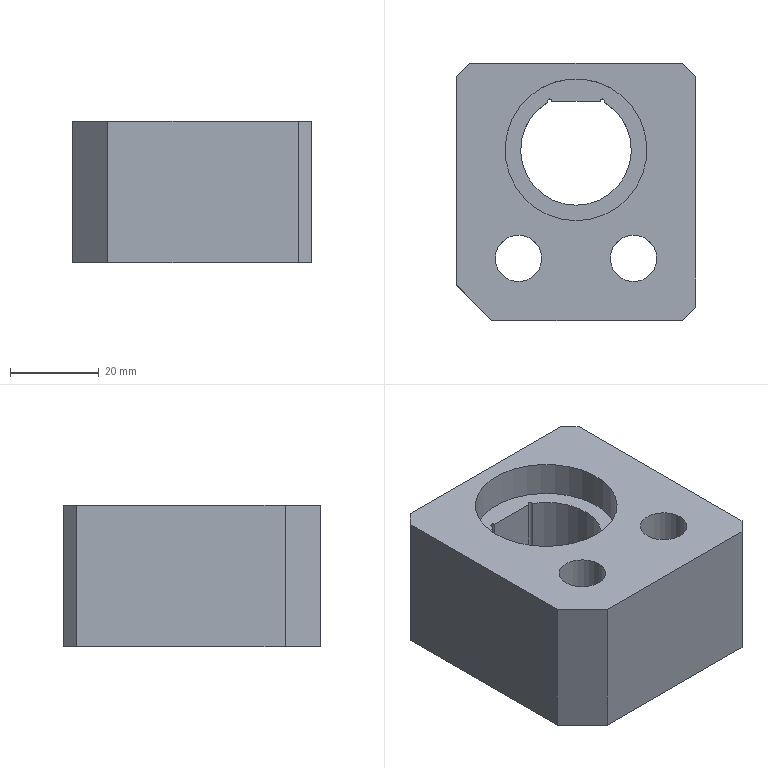Part | STEP file | lll_id3526_x_t | 1 solid | 23 faces | box 54 x 58 x 32 mm | volume 70505 mm3 | plane 14 | cylinder 9 | commonest cylinder face diameters 1 x2 10.5 x2 17 x2 25 x2 32 x1
STEP:
#1=CARTESIAN_POINT('',(3203.,139.5,84.5));
#2=VERTEX_POINT('',#1);
#3=CARTESIAN_POINT('',(3203.,155.5,84.5));
#4=DIRECTION('',(0.,0.,-1.));
#5=DIRECTION('',(1.,0.,0.));
#6=AXIS2_PLACEMENT_3D('',#3,#4,#5);
#7=CIRCLE('',#6,16.);
#8=EDGE_CURVE('',#2,#2,#7,.T.);
#9=ORIENTED_EDGE('',*,*,#8,.F.);
#10=EDGE_LOOP('',(#9));
#11=FACE_BOUND('',#10,.T.);
#12=CARTESIAN_POINT('',(3209.372,166.254,84.5));
#13=VERTEX_POINT('',#12);
#14=CARTESIAN_POINT('',(3208.437,166.5,84.5));
#15=VERTEX_POINT('',#14);
#16=CARTESIAN_POINT('',(3208.937,166.5,84.5));
#17=DIRECTION('',(0.,0.,1.));
#18=DIRECTION('',(-1.,0.,0.));
#19=AXIS2_PLACEMENT_3D('',#16,#17,#18);
#20=CIRCLE('',#19,0.5);
#21=EDGE_CURVE('',#13,#15,#20,.T.);
#22=ORIENTED_EDGE('',*,*,#21,.F.);
#23=CARTESIAN_POINT('',(3203.,143.,84.5));
#24=VERTEX_POINT('',#23);
#25=CARTESIAN_POINT('',(3203.,155.5,84.5));
#26=DIRECTION('',(0.,0.,1.));
#27=DIRECTION('',(0.,-1.,0.));
#28=AXIS2_PLACEMENT_3D('',#25,#26,#27);
#29=CIRCLE('',#28,12.5);
#30=EDGE_CURVE('',#24,#13,#29,.T.);
#31=ORIENTED_EDGE('',*,*,#30,.F.);
#32=CARTESIAN_POINT('',(3196.628,166.254,84.5));
#33=VERTEX_POINT('',#32);
#34=CARTESIAN_POINT('',(3203.,155.5,84.5));
#35=DIRECTION('',(0.,0.,1.));
#36=DIRECTION('',(0.,-1.,0.));
#37=AXIS2_PLACEMENT_3D('',#34,#35,#36);
#38=CIRCLE('',#37,12.5);
#39=EDGE_CURVE('',#33,#24,#38,.T.);
#40=ORIENTED_EDGE('',*,*,#39,.F.);
#41=CARTESIAN_POINT('',(3197.563,166.5,84.5));
#42=VERTEX_POINT('',#41);
#43=CARTESIAN_POINT('',(3197.063,166.5,84.5));
#44=DIRECTION('',(0.,0.,-1.));
#45=DIRECTION('',(1.,0.,0.));
#46=AXIS2_PLACEMENT_3D('',#43,#44,#45);
#47=CIRCLE('',#46,0.5);
#48=EDGE_CURVE('',#33,#42,#47,.T.);
#49=ORIENTED_EDGE('',*,*,#48,.T.);
#50=CARTESIAN_POINT('',(3203.,166.5,84.5));
#51=DIRECTION('',(1.,0.,0.));
#52=VECTOR('',#51,1.);
#53=LINE('',#50,#52);
#54=EDGE_CURVE('',#42,#15,#53,.T.);
#55=ORIENTED_EDGE('',*,*,#54,.T.);
#56=EDGE_LOOP('',(#22,#31,#40,#49,#55));
#57=FACE_BOUND('',#56,.T.);
#58=CARTESIAN_POINT('',(3203.,141.75,84.5));
#59=DIRECTION('',(0.,0.,-1.));
#60=DIRECTION('',(0.,-1.,0.));
#61=AXIS2_PLACEMENT_3D('',#58,#59,#60);
#62=PLANE('',#61);
#63=ADVANCED_FACE('',(#11,#57),#62,.F.);
#64=CARTESIAN_POINT('',(3210.75,131.,77.5));
#65=VERTEX_POINT('',#64);
#66=CARTESIAN_POINT('',(3216.,131.,77.5));
#67=DIRECTION('',(0.,0.,1.));
#68=DIRECTION('',(-1.,0.,0.));
#69=AXIS2_PLACEMENT_3D('',#66,#67,#68);
#70=CIRCLE('',#69,5.25);
#71=EDGE_CURVE('',#65,#65,#70,.T.);
#72=ORIENTED_EDGE('',*,*,#71,.T.);
#73=EDGE_LOOP('',(#72));
#74=FACE_BOUND('',#73,.T.);
#75=CARTESIAN_POINT('',(3207.5,131.,77.5));
#76=VERTEX_POINT('',#75);
#77=CARTESIAN_POINT('',(3216.,131.,77.5));
#78=DIRECTION('',(0.,0.,1.));
#79=DIRECTION('',(-1.,0.,0.));
#80=AXIS2_PLACEMENT_3D('',#77,#78,#79);
#81=CIRCLE('',#80,8.5);
#82=EDGE_CURVE('',#76,#76,#81,.T.);
#83=ORIENTED_EDGE('',*,*,#82,.F.);
#84=EDGE_LOOP('',(#83));
#85=FACE_BOUND('',#84,.T.);
#86=CARTESIAN_POINT('',(3216.,131.,77.5));
#87=DIRECTION('',(0.,0.,1.));
#88=DIRECTION('',(1.,0.,0.));
#89=AXIS2_PLACEMENT_3D('',#86,#87,#88);
#90=PLANE('',#89);
#91=ADVANCED_FACE('',(#74,#85),#90,.F.);
#92=ORIENTED_EDGE('',*,*,#82,.T.);
#93=EDGE_LOOP('',(#92));
#94=FACE_BOUND('',#93,.T.);
#95=CARTESIAN_POINT('',(3207.5,131.,60.5));
#96=VERTEX_POINT('',#95);
#97=CARTESIAN_POINT('',(3216.,131.,60.5));
#98=DIRECTION('',(0.,0.,-1.));
#99=DIRECTION('',(-1.,0.,0.));
#100=AXIS2_PLACEMENT_3D('',#97,#98,#99);
#101=CIRCLE('',#100,8.5);
#102=EDGE_CURVE('',#96,#96,#101,.T.);
#103=ORIENTED_EDGE('',*,*,#102,.T.);
#104=EDGE_LOOP('',(#103));
#105=FACE_BOUND('',#104,.T.);
#106=CARTESIAN_POINT('',(3216.,131.,60.5));
#107=DIRECTION('',(0.,0.,1.));
#108=DIRECTION('',(1.,0.,0.));
#109=AXIS2_PLACEMENT_3D('',#106,#107,#108);
#110=CYLINDRICAL_SURFACE('',#109,8.5);
#111=ADVANCED_FACE('',(#94,#105),#110,.F.);
#112=CARTESIAN_POINT('',(3176.,172.,60.5));
#113=VERTEX_POINT('',#112);
#114=CARTESIAN_POINT('',(3179.,175.,60.5));
#115=VERTEX_POINT('',#114);
#116=CARTESIAN_POINT('',(3196.207,192.207,60.5));
#117=DIRECTION('',(0.7071,0.7071,0.));
#118=VECTOR('',#117,1.);
#119=LINE('',#116,#118);
#120=EDGE_CURVE('',#113,#115,#119,.T.);
#121=ORIENTED_EDGE('',*,*,#120,.F.);
#122=CARTESIAN_POINT('',(3176.,172.,92.5));
#123=VERTEX_POINT('',#122);
#124=CARTESIAN_POINT('',(3176.,172.,-8.5));
#125=DIRECTION('',(0.,0.,-1.));
#126=VECTOR('',#125,1.);
#127=LINE('',#124,#126);
#128=EDGE_CURVE('',#123,#113,#127,.T.);
#129=ORIENTED_EDGE('',*,*,#128,.F.);
#130=CARTESIAN_POINT('',(3179.,175.,92.5));
#131=VERTEX_POINT('',#130);
#132=CARTESIAN_POINT('',(3196.207,192.207,92.5));
#133=DIRECTION('',(-0.7071,-0.7071,0.));
#134=VECTOR('',#133,1.);
#135=LINE('',#132,#134);
#136=EDGE_CURVE('',#131,#123,#135,.T.);
#137=ORIENTED_EDGE('',*,*,#136,.F.);
#138=CARTESIAN_POINT('',(3179.,175.,-8.5));
#139=DIRECTION('',(0.,0.,1.));
#140=VECTOR('',#139,1.);
#141=LINE('',#138,#140);
#142=EDGE_CURVE('',#115,#131,#141,.T.);
#143=ORIENTED_EDGE('',*,*,#142,.F.);
#144=EDGE_LOOP('',(#121,#129,#137,#143));
#145=FACE_OUTER_BOUND('',#144,.T.);
#146=CARTESIAN_POINT('',(3179.,175.,-8.5));
#147=DIRECTION('',(0.7071,-0.7071,0.));
#148=DIRECTION('',(0.,0.,1.));
#149=AXIS2_PLACEMENT_3D('',#146,#147,#148);
#150=PLANE('',#149);
#151=ADVANCED_FACE('',(#145),#150,.F.);
#152=CARTESIAN_POINT('',(3227.,175.,60.5));
#153=VERTEX_POINT('',#152);
#154=CARTESIAN_POINT('',(3271.14,175.,60.5));
#155=DIRECTION('',(1.,0.,0.));
#156=VECTOR('',#155,1.);
#157=LINE('',#154,#156);
#158=EDGE_CURVE('',#115,#153,#157,.T.);
#159=ORIENTED_EDGE('',*,*,#158,.F.);
#160=ORIENTED_EDGE('',*,*,#142,.T.);
#161=CARTESIAN_POINT('',(3227.,175.,92.5));
#162=VERTEX_POINT('',#161);
#163=CARTESIAN_POINT('',(3271.14,175.,92.5));
#164=DIRECTION('',(-1.,0.,0.));
#165=VECTOR('',#164,1.);
#166=LINE('',#163,#165);
#167=EDGE_CURVE('',#162,#131,#166,.T.);
#168=ORIENTED_EDGE('',*,*,#167,.F.);
#169=CARTESIAN_POINT('',(3227.,175.,-8.5));
#170=DIRECTION('',(0.,0.,-1.));
#171=VECTOR('',#170,1.);
#172=LINE('',#169,#171);
#173=EDGE_CURVE('',#162,#153,#172,.T.);
#174=ORIENTED_EDGE('',*,*,#173,.T.);
#175=EDGE_LOOP('',(#159,#160,#168,#174));
#176=FACE_OUTER_BOUND('',#175,.T.);
#177=CARTESIAN_POINT('',(3203.,175.,-8.5));
#178=DIRECTION('',(0.,1.,0.));
#179=DIRECTION('',(0.,0.,-1.));
#180=AXIS2_PLACEMENT_3D('',#177,#178,#179);
#181=PLANE('',#180);
#182=ADVANCED_FACE('',(#176),#181,.T.);
#183=CARTESIAN_POINT('',(3230.,172.,60.5));
#184=VERTEX_POINT('',#183);
#185=CARTESIAN_POINT('',(3277.933,124.067,60.5));
#186=DIRECTION('',(0.7071,-0.7071,0.));
#187=VECTOR('',#186,1.);
#188=LINE('',#185,#187);
#189=EDGE_CURVE('',#153,#184,#188,.T.);
#190=ORIENTED_EDGE('',*,*,#189,.F.);
#191=ORIENTED_EDGE('',*,*,#173,.F.);
#192=CARTESIAN_POINT('',(3230.,172.,92.5));
#193=VERTEX_POINT('',#192);
#194=CARTESIAN_POINT('',(3277.933,124.067,92.5));
#195=DIRECTION('',(-0.7071,0.7071,0.));
#196=VECTOR('',#195,1.);
#197=LINE('',#194,#196);
#198=EDGE_CURVE('',#193,#162,#197,.T.);
#199=ORIENTED_EDGE('',*,*,#198,.F.);
#200=CARTESIAN_POINT('',(3230.,172.,-8.5));
#201=DIRECTION('',(0.,0.,1.));
#202=VECTOR('',#201,1.);
#203=LINE('',#200,#202);
#204=EDGE_CURVE('',#184,#193,#203,.T.);
#205=ORIENTED_EDGE('',*,*,#204,.F.);
#206=EDGE_LOOP('',(#190,#191,#199,#205));
#207=FACE_OUTER_BOUND('',#206,.T.);
#208=CARTESIAN_POINT('',(3230.,172.,-8.5));
#209=DIRECTION('',(-0.7071,-0.7071,0.));
#210=DIRECTION('',(0.,0.,1.));
#211=AXIS2_PLACEMENT_3D('',#208,#209,#210);
#212=PLANE('',#211);
#213=ADVANCED_FACE('',(#207),#212,.F.);
#214=CARTESIAN_POINT('',(3230.,120.,92.5));
#215=VERTEX_POINT('',#214);
#216=CARTESIAN_POINT('',(3230.,124.275,92.5));
#217=DIRECTION('',(0.,1.,0.));
#218=VECTOR('',#217,1.);
#219=LINE('',#216,#218);
#220=EDGE_CURVE('',#215,#193,#219,.T.);
#221=ORIENTED_EDGE('',*,*,#220,.F.);
#222=CARTESIAN_POINT('',(3230.,120.,60.5));
#223=VERTEX_POINT('',#222);
#224=CARTESIAN_POINT('',(3230.,120.,-8.5));
#225=DIRECTION('',(0.,0.,-1.));
#226=VECTOR('',#225,1.);
#227=LINE('',#224,#226);
#228=EDGE_CURVE('',#215,#223,#227,.T.);
#229=ORIENTED_EDGE('',*,*,#228,.T.);
#230=CARTESIAN_POINT('',(3230.,124.275,60.5));
#231=DIRECTION('',(0.,-1.,0.));
#232=VECTOR('',#231,1.);
#233=LINE('',#230,#232);
#234=EDGE_CURVE('',#184,#223,#233,.T.);
#235=ORIENTED_EDGE('',*,*,#234,.F.);
#236=ORIENTED_EDGE('',*,*,#204,.T.);
#237=EDGE_LOOP('',(#221,#229,#235,#236));
#238=FACE_OUTER_BOUND('',#237,.T.);
#239=CARTESIAN_POINT('',(3230.,155.5,-8.5));
#240=DIRECTION('',(1.,0.,0.));
#241=DIRECTION('',(0.,0.,-1.));
#242=AXIS2_PLACEMENT_3D('',#239,#240,#241);
#243=PLANE('',#242);
#244=ADVANCED_FACE('',(#238),#243,.T.);
#245=CARTESIAN_POINT('',(3227.,117.,60.5));
#246=VERTEX_POINT('',#245);
#247=CARTESIAN_POINT('',(3256.207,146.207,60.5));
#248=DIRECTION('',(-0.7071,-0.7071,0.));
#249=VECTOR('',#248,1.);
#250=LINE('',#247,#249);
#251=EDGE_CURVE('',#223,#246,#250,.T.);
#252=ORIENTED_EDGE('',*,*,#251,.F.);
#253=ORIENTED_EDGE('',*,*,#228,.F.);
#254=CARTESIAN_POINT('',(3227.,117.,92.5));
#255=VERTEX_POINT('',#254);
#256=CARTESIAN_POINT('',(3256.207,146.207,92.5));
#257=DIRECTION('',(0.7071,0.7071,0.));
#258=VECTOR('',#257,1.);
#259=LINE('',#256,#258);
#260=EDGE_CURVE('',#255,#215,#259,.T.);
#261=ORIENTED_EDGE('',*,*,#260,.F.);
#262=CARTESIAN_POINT('',(3227.,117.,-8.5));
#263=DIRECTION('',(0.,0.,1.));
#264=VECTOR('',#263,1.);
#265=LINE('',#262,#264);
#266=EDGE_CURVE('',#246,#255,#265,.T.);
#267=ORIENTED_EDGE('',*,*,#266,.F.);
#268=EDGE_LOOP('',(#252,#253,#261,#267));
#269=FACE_OUTER_BOUND('',#268,.T.);
#270=CARTESIAN_POINT('',(3227.,117.,-8.5));
#271=DIRECTION('',(-0.7071,0.7071,0.));
#272=DIRECTION('',(0.,0.,1.));
#273=AXIS2_PLACEMENT_3D('',#270,#271,#272);
#274=PLANE('',#273);
#275=ADVANCED_FACE('',(#269),#274,.F.);
#276=CARTESIAN_POINT('',(3184.,117.,92.5));
#277=VERTEX_POINT('',#276);
#278=CARTESIAN_POINT('',(3271.14,117.,92.5));
#279=DIRECTION('',(1.,0.,0.));
#280=VECTOR('',#279,1.);
#281=LINE('',#278,#280);
#282=EDGE_CURVE('',#277,#255,#281,.T.);
#283=ORIENTED_EDGE('',*,*,#282,.F.);
#284=CARTESIAN_POINT('',(3184.,117.,60.5));
#285=VERTEX_POINT('',#284);
#286=CARTESIAN_POINT('',(3184.,117.,-8.5));
#287=DIRECTION('',(0.,0.,-1.));
#288=VECTOR('',#287,1.);
#289=LINE('',#286,#288);
#290=EDGE_CURVE('',#277,#285,#289,.T.);
#291=ORIENTED_EDGE('',*,*,#290,.T.);
#292=CARTESIAN_POINT('',(3271.14,117.,60.5));
#293=DIRECTION('',(-1.,0.,0.));
#294=VECTOR('',#293,1.);
#295=LINE('',#292,#294);
#296=EDGE_CURVE('',#246,#285,#295,.T.);
#297=ORIENTED_EDGE('',*,*,#296,.F.);
#298=ORIENTED_EDGE('',*,*,#266,.T.);
#299=EDGE_LOOP('',(#283,#291,#297,#298));
#300=FACE_OUTER_BOUND('',#299,.T.);
#301=CARTESIAN_POINT('',(3203.,117.,-8.5));
#302=DIRECTION('',(0.,-1.,0.));
#303=DIRECTION('',(0.,0.,1.));
#304=AXIS2_PLACEMENT_3D('',#301,#302,#303);
#305=PLANE('',#304);
#306=ADVANCED_FACE('',(#300),#305,.T.);
#307=CARTESIAN_POINT('',(3176.,125.,60.5));
#308=VERTEX_POINT('',#307);
#309=CARTESIAN_POINT('',(3220.433,80.567,60.5));
#310=DIRECTION('',(-0.7071,0.7071,0.));
#311=VECTOR('',#310,1.);
#312=LINE('',#309,#311);
#313=EDGE_CURVE('',#285,#308,#312,.T.);
#314=ORIENTED_EDGE('',*,*,#313,.F.);
#315=ORIENTED_EDGE('',*,*,#290,.F.);
#316=CARTESIAN_POINT('',(3176.,125.,92.5));
#317=VERTEX_POINT('',#316);
#318=CARTESIAN_POINT('',(3220.433,80.567,92.5));
#319=DIRECTION('',(0.7071,-0.7071,0.));
#320=VECTOR('',#319,1.);
#321=LINE('',#318,#320);
#322=EDGE_CURVE('',#317,#277,#321,.T.);
#323=ORIENTED_EDGE('',*,*,#322,.F.);
#324=CARTESIAN_POINT('',(3176.,125.,-8.5));
#325=DIRECTION('',(0.,0.,1.));
#326=VECTOR('',#325,1.);
#327=LINE('',#324,#326);
#328=EDGE_CURVE('',#308,#317,#327,.T.);
#329=ORIENTED_EDGE('',*,*,#328,.F.);
#330=EDGE_LOOP('',(#314,#315,#323,#329));
#331=FACE_OUTER_BOUND('',#330,.T.);
#332=CARTESIAN_POINT('',(3176.,125.,-8.5));
#333=DIRECTION('',(0.7071,0.7071,0.));
#334=DIRECTION('',(0.,0.,1.));
#335=AXIS2_PLACEMENT_3D('',#332,#333,#334);
#336=PLANE('',#335);
#337=ADVANCED_FACE('',(#331),#336,.F.);
#338=CARTESIAN_POINT('',(3176.,124.275,60.5));
#339=DIRECTION('',(0.,1.,0.));
#340=VECTOR('',#339,1.);
#341=LINE('',#338,#340);
#342=EDGE_CURVE('',#308,#113,#341,.T.);
#343=ORIENTED_EDGE('',*,*,#342,.F.);
#344=ORIENTED_EDGE('',*,*,#328,.T.);
#345=CARTESIAN_POINT('',(3176.,124.275,92.5));
#346=DIRECTION('',(0.,-1.,0.));
#347=VECTOR('',#346,1.);
#348=LINE('',#345,#347);
#349=EDGE_CURVE('',#123,#317,#348,.T.);
#350=ORIENTED_EDGE('',*,*,#349,.F.);
#351=ORIENTED_EDGE('',*,*,#128,.T.);
#352=EDGE_LOOP('',(#343,#344,#350,#351));
#353=FACE_OUTER_BOUND('',#352,.T.);
#354=CARTESIAN_POINT('',(3176.,155.5,-8.5));
#355=DIRECTION('',(-1.,0.,0.));
#356=DIRECTION('',(0.,0.,1.));
#357=AXIS2_PLACEMENT_3D('',#354,#355,#356);
#358=PLANE('',#357);
#359=ADVANCED_FACE('',(#353),#358,.T.);
#360=CARTESIAN_POINT('',(3210.75,131.,92.5));
#361=VERTEX_POINT('',#360);
#362=CARTESIAN_POINT('',(3216.,131.,92.5));
#363=DIRECTION('',(0.,0.,-1.));
#364=DIRECTION('',(-1.,0.,0.));
#365=AXIS2_PLACEMENT_3D('',#362,#363,#364);
#366=CIRCLE('',#365,5.25);
#367=EDGE_CURVE('',#361,#361,#366,.T.);
#368=ORIENTED_EDGE('',*,*,#367,.F.);
#369=EDGE_LOOP('',(#368));
#370=FACE_BOUND('',#369,.T.);
#371=ORIENTED_EDGE('',*,*,#71,.F.);
#372=EDGE_LOOP('',(#371));
#373=FACE_BOUND('',#372,.T.);
#374=CARTESIAN_POINT('',(3216.,131.,160.5));
#375=DIRECTION('',(0.,0.,1.));
#376=DIRECTION('',(1.,0.,0.));
#377=AXIS2_PLACEMENT_3D('',#374,#375,#376);
#378=CYLINDRICAL_SURFACE('',#377,5.25);
#379=ADVANCED_FACE('',(#370,#373),#378,.F.);
#380=CARTESIAN_POINT('',(3203.,139.5,92.5));
#381=VERTEX_POINT('',#380);
#382=CARTESIAN_POINT('',(3203.,155.5,92.5));
#383=DIRECTION('',(0.,0.,1.));
#384=DIRECTION('',(-1.,0.,0.));
#385=AXIS2_PLACEMENT_3D('',#382,#383,#384);
#386=CIRCLE('',#385,16.);
#387=EDGE_CURVE('',#381,#381,#386,.T.);
#388=ORIENTED_EDGE('',*,*,#387,.T.);
#389=CARTESIAN_POINT('',(3203.,139.5,88.5));
#390=DIRECTION('',(0.,0.,-1.));
#391=VECTOR('',#390,1.);
#392=LINE('',#389,#391);
#393=EDGE_CURVE('',#381,#2,#392,.T.);
#394=ORIENTED_EDGE('',*,*,#393,.T.);
#395=ORIENTED_EDGE('',*,*,#8,.T.);
#396=ORIENTED_EDGE('',*,*,#393,.F.);
#397=EDGE_LOOP('',(#388,#394,#395,#396));
#398=FACE_OUTER_BOUND('',#397,.T.);
#399=CARTESIAN_POINT('',(3203.,155.5,88.5));
#400=DIRECTION('',(0.,0.,-1.));
#401=DIRECTION('',(0.,1.,0.));
#402=AXIS2_PLACEMENT_3D('',#399,#400,#401);
#403=CYLINDRICAL_SURFACE('',#402,16.);
#404=ADVANCED_FACE('',(#398),#403,.F.);
#405=CARTESIAN_POINT('',(3195.25,131.,92.5));
#406=VERTEX_POINT('',#405);
#407=CARTESIAN_POINT('',(3190.,131.,92.5));
#408=DIRECTION('',(0.,0.,1.));
#409=DIRECTION('',(1.,0.,0.));
#410=AXIS2_PLACEMENT_3D('',#407,#408,#409);
#411=CIRCLE('',#410,5.25);
#412=EDGE_CURVE('',#406,#406,#411,.T.);
#413=ORIENTED_EDGE('',*,*,#412,.F.);
#414=EDGE_LOOP('',(#413));
#415=FACE_BOUND('',#414,.T.);
#416=ORIENTED_EDGE('',*,*,#387,.F.);
#417=EDGE_LOOP('',(#416));
#418=FACE_BOUND('',#417,.T.);
#419=ORIENTED_EDGE('',*,*,#367,.T.);
#420=EDGE_LOOP('',(#419));
#421=FACE_BOUND('',#420,.T.);
#422=ORIENTED_EDGE('',*,*,#349,.T.);
#423=ORIENTED_EDGE('',*,*,#322,.T.);
#424=ORIENTED_EDGE('',*,*,#282,.T.);
#425=ORIENTED_EDGE('',*,*,#260,.T.);
#426=ORIENTED_EDGE('',*,*,#220,.T.);
#427=ORIENTED_EDGE('',*,*,#198,.T.);
#428=ORIENTED_EDGE('',*,*,#167,.T.);
#429=ORIENTED_EDGE('',*,*,#136,.T.);
#430=EDGE_LOOP('',(#422,#423,#424,#425,#426,#427,#428,#429));
#431=FACE_BOUND('',#430,.T.);
#432=CARTESIAN_POINT('',(3271.14,124.275,92.5));
#433=DIRECTION('',(0.,0.,1.));
#434=DIRECTION('',(1.,0.,0.));
#435=AXIS2_PLACEMENT_3D('',#432,#433,#434);
#436=PLANE('',#435);
#437=ADVANCED_FACE('',(#415,#418,#421,#431),#436,.T.);
#438=CARTESIAN_POINT('',(3208.437,166.5,60.5));
#439=VERTEX_POINT('',#438);
#440=CARTESIAN_POINT('',(3209.372,166.254,60.5));
#441=VERTEX_POINT('',#440);
#442=CARTESIAN_POINT('',(3208.937,166.5,60.5));
#443=DIRECTION('',(0.,0.,-1.));
#444=DIRECTION('',(1.,0.,0.));
#445=AXIS2_PLACEMENT_3D('',#442,#443,#444);
#446=CIRCLE('',#445,0.5);
#447=EDGE_CURVE('',#439,#441,#446,.T.);
#448=ORIENTED_EDGE('',*,*,#447,.F.);
#449=CARTESIAN_POINT('',(3197.563,166.5,60.5));
#450=VERTEX_POINT('',#449);
#451=CARTESIAN_POINT('',(3271.14,166.5,60.5));
#452=DIRECTION('',(1.,0.,0.));
#453=VECTOR('',#452,1.);
#454=LINE('',#451,#453);
#455=EDGE_CURVE('',#450,#439,#454,.T.);
#456=ORIENTED_EDGE('',*,*,#455,.F.);
#457=CARTESIAN_POINT('',(3196.628,166.254,60.5));
#458=VERTEX_POINT('',#457);
#459=CARTESIAN_POINT('',(3197.063,166.5,60.5));
#460=DIRECTION('',(0.,0.,-1.));
#461=DIRECTION('',(1.,0.,0.));
#462=AXIS2_PLACEMENT_3D('',#459,#460,#461);
#463=CIRCLE('',#462,0.5);
#464=EDGE_CURVE('',#458,#450,#463,.T.);
#465=ORIENTED_EDGE('',*,*,#464,.F.);
#466=CARTESIAN_POINT('',(3203.,143.,60.5));
#467=VERTEX_POINT('',#466);
#468=CARTESIAN_POINT('',(3203.,155.5,60.5));
#469=DIRECTION('',(0.,0.,-1.));
#470=DIRECTION('',(1.,0.,0.));
#471=AXIS2_PLACEMENT_3D('',#468,#469,#470);
#472=CIRCLE('',#471,12.5);
#473=EDGE_CURVE('',#467,#458,#472,.T.);
#474=ORIENTED_EDGE('',*,*,#473,.F.);
#475=CARTESIAN_POINT('',(3203.,155.5,60.5));
#476=DIRECTION('',(0.,0.,-1.));
#477=DIRECTION('',(1.,0.,0.));
#478=AXIS2_PLACEMENT_3D('',#475,#476,#477);
#479=CIRCLE('',#478,12.5);
#480=EDGE_CURVE('',#441,#467,#479,.T.);
#481=ORIENTED_EDGE('',*,*,#480,.F.);
#482=EDGE_LOOP('',(#448,#456,#465,#474,#481));
#483=FACE_BOUND('',#482,.T.);
#484=CARTESIAN_POINT('',(3198.5,131.,60.5));
#485=VERTEX_POINT('',#484);
#486=CARTESIAN_POINT('',(3190.,131.,60.5));
#487=DIRECTION('',(0.,0.,-1.));
#488=DIRECTION('',(1.,0.,0.));
#489=AXIS2_PLACEMENT_3D('',#486,#487,#488);
#490=CIRCLE('',#489,8.5);
#491=EDGE_CURVE('',#485,#485,#490,.T.);
#492=ORIENTED_EDGE('',*,*,#491,.F.);
#493=EDGE_LOOP('',(#492));
#494=FACE_BOUND('',#493,.T.);
#495=ORIENTED_EDGE('',*,*,#296,.T.);
#496=ORIENTED_EDGE('',*,*,#313,.T.);
#497=ORIENTED_EDGE('',*,*,#342,.T.);
#498=ORIENTED_EDGE('',*,*,#120,.T.);
#499=ORIENTED_EDGE('',*,*,#158,.T.);
#500=ORIENTED_EDGE('',*,*,#189,.T.);
#501=ORIENTED_EDGE('',*,*,#234,.T.);
#502=ORIENTED_EDGE('',*,*,#251,.T.);
#503=EDGE_LOOP('',(#495,#496,#497,#498,#499,#500,#501,#502));
#504=FACE_BOUND('',#503,.T.);
#505=ORIENTED_EDGE('',*,*,#102,.F.);
#506=EDGE_LOOP('',(#505));
#507=FACE_BOUND('',#506,.T.);
#508=CARTESIAN_POINT('',(3271.14,124.275,60.5));
#509=DIRECTION('',(0.,0.,1.));
#510=DIRECTION('',(1.,0.,0.));
#511=AXIS2_PLACEMENT_3D('',#508,#509,#510);
#512=PLANE('',#511);
#513=ADVANCED_FACE('',(#483,#494,#504,#507),#512,.F.);
#514=CARTESIAN_POINT('',(3195.25,131.,77.5));
#515=VERTEX_POINT('',#514);
#516=CARTESIAN_POINT('',(3190.,131.,77.5));
#517=DIRECTION('',(0.,0.,1.));
#518=DIRECTION('',(1.,0.,0.));
#519=AXIS2_PLACEMENT_3D('',#516,#517,#518);
#520=CIRCLE('',#519,5.25);
#521=EDGE_CURVE('',#515,#515,#520,.T.);
#522=ORIENTED_EDGE('',*,*,#521,.T.);
#523=EDGE_LOOP('',(#522));
#524=FACE_BOUND('',#523,.T.);
#525=CARTESIAN_POINT('',(3198.5,131.,77.5));
#526=VERTEX_POINT('',#525);
#527=CARTESIAN_POINT('',(3190.,131.,77.5));
#528=DIRECTION('',(0.,0.,1.));
#529=DIRECTION('',(1.,0.,0.));
#530=AXIS2_PLACEMENT_3D('',#527,#528,#529);
#531=CIRCLE('',#530,8.5);
#532=EDGE_CURVE('',#526,#526,#531,.T.);
#533=ORIENTED_EDGE('',*,*,#532,.F.);
#534=EDGE_LOOP('',(#533));
#535=FACE_BOUND('',#534,.T.);
#536=CARTESIAN_POINT('',(3190.,131.,77.5));
#537=DIRECTION('',(0.,0.,1.));
#538=DIRECTION('',(-1.,0.,0.));
#539=AXIS2_PLACEMENT_3D('',#536,#537,#538);
#540=PLANE('',#539);
#541=ADVANCED_FACE('',(#524,#535),#540,.F.);
#542=ORIENTED_EDGE('',*,*,#412,.T.);
#543=EDGE_LOOP('',(#542));
#544=FACE_BOUND('',#543,.T.);
#545=ORIENTED_EDGE('',*,*,#521,.F.);
#546=EDGE_LOOP('',(#545));
#547=FACE_BOUND('',#546,.T.);
#548=CARTESIAN_POINT('',(3190.,131.,160.5));
#549=DIRECTION('',(0.,0.,1.));
#550=DIRECTION('',(-1.,0.,0.));
#551=AXIS2_PLACEMENT_3D('',#548,#549,#550);
#552=CYLINDRICAL_SURFACE('',#551,5.25);
#553=ADVANCED_FACE('',(#544,#547),#552,.F.);
#554=ORIENTED_EDGE('',*,*,#532,.T.);
#555=EDGE_LOOP('',(#554));
#556=FACE_BOUND('',#555,.T.);
#557=ORIENTED_EDGE('',*,*,#491,.T.);
#558=EDGE_LOOP('',(#557));
#559=FACE_BOUND('',#558,.T.);
#560=CARTESIAN_POINT('',(3190.,131.,60.5));
#561=DIRECTION('',(0.,0.,1.));
#562=DIRECTION('',(-1.,0.,0.));
#563=AXIS2_PLACEMENT_3D('',#560,#561,#562);
#564=CYLINDRICAL_SURFACE('',#563,8.5);
#565=ADVANCED_FACE('',(#556,#559),#564,.F.);
#566=ORIENTED_EDGE('',*,*,#455,.T.);
#567=CARTESIAN_POINT('',(3208.437,166.5,84.5));
#568=DIRECTION('',(0.,0.,1.));
#569=VECTOR('',#568,1.);
#570=LINE('',#567,#569);
#571=EDGE_CURVE('',#439,#15,#570,.T.);
#572=ORIENTED_EDGE('',*,*,#571,.T.);
#573=ORIENTED_EDGE('',*,*,#54,.F.);
#574=CARTESIAN_POINT('',(3197.563,166.5,84.5));
#575=DIRECTION('',(0.,0.,-1.));
#576=VECTOR('',#575,1.);
#577=LINE('',#574,#576);
#578=EDGE_CURVE('',#42,#450,#577,.T.);
#579=ORIENTED_EDGE('',*,*,#578,.T.);
#580=EDGE_LOOP('',(#566,#572,#573,#579));
#581=FACE_OUTER_BOUND('',#580,.T.);
#582=CARTESIAN_POINT('',(3203.,166.5,56.341));
#583=DIRECTION('',(0.,1.,0.));
#584=DIRECTION('',(0.,0.,1.));
#585=AXIS2_PLACEMENT_3D('',#582,#583,#584);
#586=PLANE('',#585);
#587=ADVANCED_FACE('',(#581),#586,.F.);
#588=ORIENTED_EDGE('',*,*,#30,.T.);
#589=CARTESIAN_POINT('',(3209.372,166.254,67.));
#590=DIRECTION('',(0.,0.,-1.));
#591=VECTOR('',#590,1.);
#592=LINE('',#589,#591);
#593=EDGE_CURVE('',#13,#441,#592,.T.);
#594=ORIENTED_EDGE('',*,*,#593,.T.);
#595=ORIENTED_EDGE('',*,*,#480,.T.);
#596=CARTESIAN_POINT('',(3203.,143.,38.5));
#597=DIRECTION('',(0.,0.,-1.));
#598=VECTOR('',#597,1.);
#599=LINE('',#596,#598);
#600=EDGE_CURVE('',#24,#467,#599,.T.);
#601=ORIENTED_EDGE('',*,*,#600,.F.);
#602=EDGE_LOOP('',(#588,#594,#595,#601));
#603=FACE_OUTER_BOUND('',#602,.T.);
#604=CARTESIAN_POINT('',(3203.,155.5,38.5));
#605=DIRECTION('',(0.,0.,-1.));
#606=DIRECTION('',(0.,1.,0.));
#607=AXIS2_PLACEMENT_3D('',#604,#605,#606);
#608=CYLINDRICAL_SURFACE('',#607,12.5);
#609=ADVANCED_FACE('',(#603),#608,.F.);
#610=ORIENTED_EDGE('',*,*,#473,.T.);
#611=CARTESIAN_POINT('',(3196.628,166.254,67.));
#612=DIRECTION('',(0.,0.,1.));
#613=VECTOR('',#612,1.);
#614=LINE('',#611,#613);
#615=EDGE_CURVE('',#458,#33,#614,.T.);
#616=ORIENTED_EDGE('',*,*,#615,.T.);
#617=ORIENTED_EDGE('',*,*,#39,.T.);
#618=ORIENTED_EDGE('',*,*,#600,.T.);
#619=EDGE_LOOP('',(#610,#616,#617,#618));
#620=FACE_OUTER_BOUND('',#619,.T.);
#621=CARTESIAN_POINT('',(3203.,155.5,38.5));
#622=DIRECTION('',(0.,0.,-1.));
#623=DIRECTION('',(0.,1.,0.));
#624=AXIS2_PLACEMENT_3D('',#621,#622,#623);
#625=CYLINDRICAL_SURFACE('',#624,12.5);
#626=ADVANCED_FACE('',(#620),#625,.F.);
#627=ORIENTED_EDGE('',*,*,#48,.F.);
#628=ORIENTED_EDGE('',*,*,#615,.F.);
#629=ORIENTED_EDGE('',*,*,#464,.T.);
#630=ORIENTED_EDGE('',*,*,#578,.F.);
#631=EDGE_LOOP('',(#627,#628,#629,#630));
#632=FACE_OUTER_BOUND('',#631,.T.);
#633=CARTESIAN_POINT('',(3197.063,166.5,84.5));
#634=DIRECTION('',(0.,0.,-1.));
#635=DIRECTION('',(1.,0.,0.));
#636=AXIS2_PLACEMENT_3D('',#633,#634,#635);
#637=CYLINDRICAL_SURFACE('',#636,0.5);
#638=ADVANCED_FACE('',(#632),#637,.F.);
#639=ORIENTED_EDGE('',*,*,#447,.T.);
#640=ORIENTED_EDGE('',*,*,#593,.F.);
#641=ORIENTED_EDGE('',*,*,#21,.T.);
#642=ORIENTED_EDGE('',*,*,#571,.F.);
#643=EDGE_LOOP('',(#639,#640,#641,#642));
#644=FACE_OUTER_BOUND('',#643,.T.);
#645=CARTESIAN_POINT('',(3208.937,166.5,84.5));
#646=DIRECTION('',(0.,0.,-1.));
#647=DIRECTION('',(-1.,0.,0.));
#648=AXIS2_PLACEMENT_3D('',#645,#646,#647);
#649=CYLINDRICAL_SURFACE('',#648,0.5);
#650=ADVANCED_FACE('',(#644),#649,.F.);
#651=CLOSED_SHELL('',(#63,#91,#111,#151,#182,#213,#244,#275,#306,#337,#359,#379,#404,#437,#513,#541,#553,#565,#587,#609,#626,#638,#650));
#652=MANIFOLD_SOLID_BREP('',#651);
#653=(LENGTH_UNIT()NAMED_UNIT(*)SI_UNIT(.MILLI.,.METRE.));
#654=UNCERTAINTY_MEASURE_WITH_UNIT(LENGTH_MEASURE(0.00002),#653,'','');
#655=(NAMED_UNIT(*)PLANE_ANGLE_UNIT()SI_UNIT($,.RADIAN.));
#656=PLANE_ANGLE_MEASURE_WITH_UNIT(PLANE_ANGLE_MEASURE(0.01745),#655);
#657=DIMENSIONAL_EXPONENTS(0.,0.,0.,0.,0.,0.,0.);
#658=(CONVERSION_BASED_UNIT('DEGREE',#656)NAMED_UNIT(#657)PLANE_ANGLE_UNIT());
#659=(NAMED_UNIT(*)SI_UNIT($,.STERADIAN.)SOLID_ANGLE_UNIT());
#660=(GEOMETRIC_REPRESENTATION_CONTEXT(3)GLOBAL_UNCERTAINTY_ASSIGNED_CONTEXT((#654))GLOBAL_UNIT_ASSIGNED_CONTEXT((#653,#658,#659))REPRESENTATION_CONTEXT('',''));
#661=ADVANCED_BREP_SHAPE_REPRESENTATION('',(#652),#660);